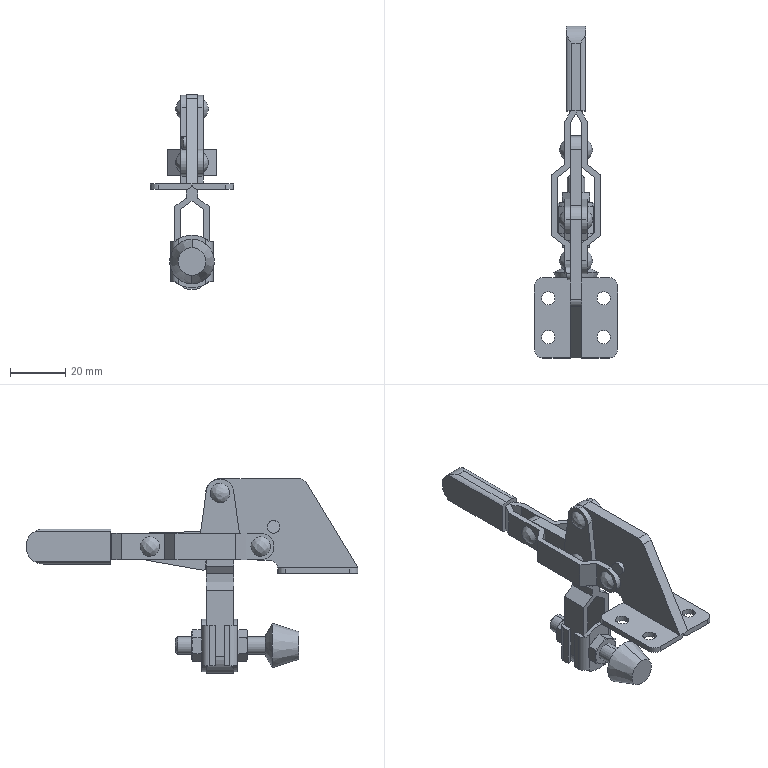Part | SolidWorks | features LocalCirPattern 1, ReferencePattern 1 | 5 solids | 248 faces | box 30 x 119.8 x 70.25 mm | volume 20145 mm3 | plane 128 | cylinder 79 | cone 33 | spline 8 | commonest cylinder face diameters 4.8 x24 6 x9 10 x8 6.35 x6 19 x6 2.5 x4